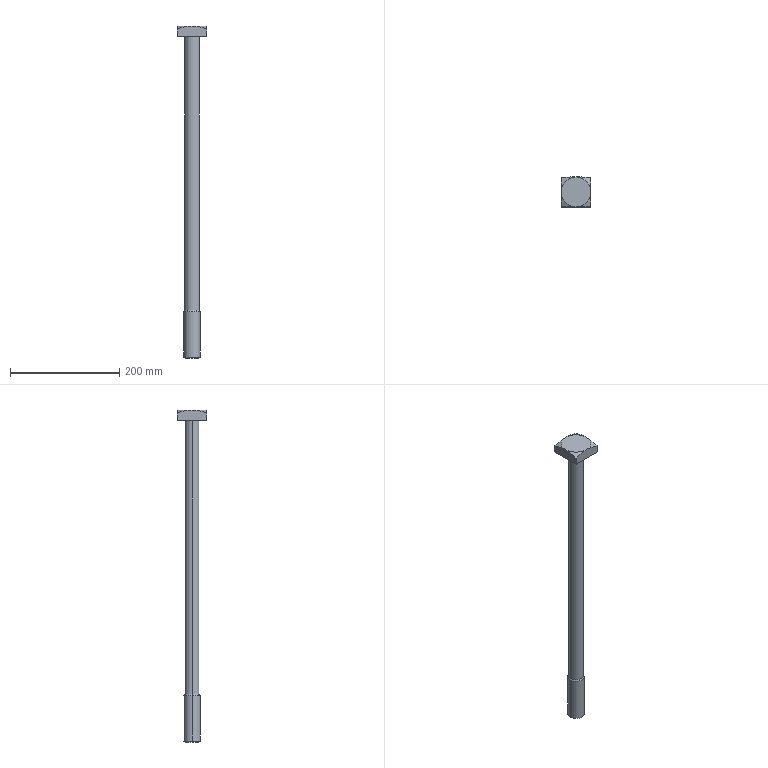Part | SolidWorks | features Cut 1, Extrusion 1, Fillet 1, LPattern 1, RevCut 1, Revolution 1 | 1 solid | 21 faces | box 55 x 55 x 609 mm | volume 405608 mm3 | cone 8 | plane 7 | cylinder 4 | torus 2 | commonest cylinder face diameters 27 x2 30 x2
STEP:
#1=CARTESIAN_POINT('',(11.969,0.,-590.));
#2=VERTEX_POINT('',#1);
#3=CARTESIAN_POINT('',(-11.969,0.,-590.));
#4=VERTEX_POINT('',#3);
#5=CARTESIAN_POINT('',(0.,0.,-590.));
#6=DIRECTION('',(0.,0.,1.));
#7=DIRECTION('',(1.,0.,0.));
#8=AXIS2_PLACEMENT_3D('',#5,#6,#7);
#9=CIRCLE('',#8,11.969);
#10=EDGE_CURVE('',#2,#4,#9,.T.);
#11=ORIENTED_EDGE('',*,*,#10,.T.);
#12=CARTESIAN_POINT('',(-15.,0.,-588.25));
#13=VERTEX_POINT('',#12);
#14=CARTESIAN_POINT('',(-11.969,0.,-590.));
#15=DIRECTION('',(-0.866,0.,0.5));
#16=VECTOR('',#15,1000.);
#17=LINE('',#14,#16);
#18=EDGE_CURVE('',#4,#13,#17,.T.);
#19=ORIENTED_EDGE('',*,*,#18,.T.);
#20=CARTESIAN_POINT('',(15.,0.,-588.25));
#21=VERTEX_POINT('',#20);
#22=CARTESIAN_POINT('',(0.,0.,-588.25));
#23=DIRECTION('',(0.,0.,1.));
#24=DIRECTION('',(1.,0.,0.));
#25=AXIS2_PLACEMENT_3D('',#22,#23,#24);
#26=CIRCLE('',#25,15.);
#27=EDGE_CURVE('',#21,#13,#26,.T.);
#28=ORIENTED_EDGE('',*,*,#27,.F.);
#29=CARTESIAN_POINT('',(11.969,0.,-590.));
#30=DIRECTION('',(0.866,0.,0.5));
#31=VECTOR('',#30,1000.);
#32=LINE('',#29,#31);
#33=EDGE_CURVE('',#2,#21,#32,.T.);
#34=ORIENTED_EDGE('',*,*,#33,.F.);
#35=EDGE_LOOP('',(#11,#19,#28,#34));
#36=FACE_OUTER_BOUND('',#35,.T.);
#37=CARTESIAN_POINT('',(0.,0.,-590.));
#38=DIRECTION('',(0.,0.,1.));
#39=DIRECTION('',(1.,0.,0.));
#40=AXIS2_PLACEMENT_3D('',#37,#38,#39);
#41=CONICAL_SURFACE('',#40,11.969,1.047);
#42=ADVANCED_FACE('',(#36),#41,.T.);
#43=CARTESIAN_POINT('',(-14.5,0.,0.));
#44=VERTEX_POINT('',#43);
#45=CARTESIAN_POINT('',(14.5,0.,0.));
#46=VERTEX_POINT('',#45);
#47=CARTESIAN_POINT('',(0.,0.,0.));
#48=DIRECTION('',(0.,0.,1.));
#49=DIRECTION('',(1.,0.,0.));
#50=AXIS2_PLACEMENT_3D('',#47,#48,#49);
#51=CIRCLE('',#50,14.5);
#52=EDGE_CURVE('',#44,#46,#51,.T.);
#53=ORIENTED_EDGE('',*,*,#52,.F.);
#54=CARTESIAN_POINT('',(-13.5,0.,-1.));
#55=VERTEX_POINT('',#54);
#56=CARTESIAN_POINT('',(-14.5,0.,-1.));
#57=DIRECTION('',(0.,1.,0.));
#58=DIRECTION('',(-1.,0.,0.));
#59=AXIS2_PLACEMENT_3D('',#56,#57,#58);
#60=CIRCLE('',#59,1.);
#61=EDGE_CURVE('',#44,#55,#60,.T.);
#62=ORIENTED_EDGE('',*,*,#61,.T.);
#63=CARTESIAN_POINT('',(13.5,0.,-1.));
#64=VERTEX_POINT('',#63);
#65=CARTESIAN_POINT('',(0.,0.,-1.));
#66=DIRECTION('',(0.,0.,-1.));
#67=DIRECTION('',(1.,0.,0.));
#68=AXIS2_PLACEMENT_3D('',#65,#66,#67);
#69=CIRCLE('',#68,13.5);
#70=EDGE_CURVE('',#64,#55,#69,.T.);
#71=ORIENTED_EDGE('',*,*,#70,.F.);
#72=CARTESIAN_POINT('',(14.5,0.,-1.));
#73=DIRECTION('',(0.,-1.,0.));
#74=DIRECTION('',(0.,0.,-1.));
#75=AXIS2_PLACEMENT_3D('',#72,#73,#74);
#76=CIRCLE('',#75,1.);
#77=EDGE_CURVE('',#46,#64,#76,.T.);
#78=ORIENTED_EDGE('',*,*,#77,.F.);
#79=EDGE_LOOP('',(#53,#62,#71,#78));
#80=FACE_OUTER_BOUND('',#79,.T.);
#81=CARTESIAN_POINT('',(0.,0.,-1.));
#82=DIRECTION('',(0.,0.,1.));
#83=DIRECTION('',(1.,0.,0.));
#84=AXIS2_PLACEMENT_3D('',#81,#82,#83);
#85=TOROIDAL_SURFACE('',#84,14.5,1.);
#86=ADVANCED_FACE('',(#80),#85,.F.);
#87=CARTESIAN_POINT('',(-15.,0.,-505.));
#88=VERTEX_POINT('',#87);
#89=CARTESIAN_POINT('',(15.,0.,-505.));
#90=VERTEX_POINT('',#89);
#91=CARTESIAN_POINT('',(0.,0.,-505.));
#92=DIRECTION('',(0.,0.,-1.));
#93=DIRECTION('',(-1.,0.,0.));
#94=AXIS2_PLACEMENT_3D('',#91,#92,#93);
#95=CIRCLE('',#94,15.);
#96=EDGE_CURVE('',#88,#90,#95,.T.);
#97=ORIENTED_EDGE('',*,*,#96,.T.);
#98=CARTESIAN_POINT('',(15.,0.,-590.));
#99=DIRECTION('',(0.,0.,-1.));
#100=VECTOR('',#99,1000.);
#101=LINE('',#98,#100);
#102=EDGE_CURVE('',#90,#21,#101,.T.);
#103=ORIENTED_EDGE('',*,*,#102,.T.);
#104=ORIENTED_EDGE('',*,*,#27,.T.);
#105=CARTESIAN_POINT('',(-15.,0.,-590.));
#106=DIRECTION('',(0.,0.,-1.));
#107=VECTOR('',#106,1000.);
#108=LINE('',#105,#107);
#109=EDGE_CURVE('',#88,#13,#108,.T.);
#110=ORIENTED_EDGE('',*,*,#109,.F.);
#111=EDGE_LOOP('',(#97,#103,#104,#110));
#112=FACE_OUTER_BOUND('',#111,.T.);
#113=CARTESIAN_POINT('',(0.,0.,-590.));
#114=DIRECTION('',(0.,0.,-1.));
#115=DIRECTION('',(-1.,0.,0.));
#116=AXIS2_PLACEMENT_3D('',#113,#114,#115);
#117=CYLINDRICAL_SURFACE('',#116,15.);
#118=ADVANCED_FACE('',(#112),#117,.T.);
#119=CARTESIAN_POINT('',(-13.5,0.,-502.402));
#120=VERTEX_POINT('',#119);
#121=CARTESIAN_POINT('',(13.5,0.,-502.402));
#122=VERTEX_POINT('',#121);
#123=CARTESIAN_POINT('',(0.,0.,-502.402));
#124=DIRECTION('',(0.,0.,-1.));
#125=DIRECTION('',(-1.,0.,0.));
#126=AXIS2_PLACEMENT_3D('',#123,#124,#125);
#127=CIRCLE('',#126,13.5);
#128=EDGE_CURVE('',#120,#122,#127,.T.);
#129=ORIENTED_EDGE('',*,*,#128,.T.);
#130=CARTESIAN_POINT('',(13.5,0.,-502.402));
#131=DIRECTION('',(0.5,0.,-0.866));
#132=VECTOR('',#131,1000.);
#133=LINE('',#130,#132);
#134=EDGE_CURVE('',#122,#90,#133,.T.);
#135=ORIENTED_EDGE('',*,*,#134,.T.);
#136=ORIENTED_EDGE('',*,*,#96,.F.);
#137=CARTESIAN_POINT('',(-13.5,0.,-502.402));
#138=DIRECTION('',(-0.5,0.,-0.866));
#139=VECTOR('',#138,1000.);
#140=LINE('',#137,#139);
#141=EDGE_CURVE('',#120,#88,#140,.T.);
#142=ORIENTED_EDGE('',*,*,#141,.F.);
#143=EDGE_LOOP('',(#129,#135,#136,#142));
#144=FACE_OUTER_BOUND('',#143,.T.);
#145=CARTESIAN_POINT('',(0.,0.,-502.402));
#146=DIRECTION('',(0.,0.,-1.));
#147=DIRECTION('',(-1.,0.,0.));
#148=AXIS2_PLACEMENT_3D('',#145,#146,#147);
#149=CONICAL_SURFACE('',#148,13.5,0.5236);
#150=ADVANCED_FACE('',(#144),#149,.T.);
#151=CARTESIAN_POINT('',(0.,0.,-1.));
#152=DIRECTION('',(0.,0.,-1.));
#153=DIRECTION('',(1.,0.,0.));
#154=AXIS2_PLACEMENT_3D('',#151,#152,#153);
#155=CIRCLE('',#154,13.5);
#156=EDGE_CURVE('',#55,#64,#155,.T.);
#157=ORIENTED_EDGE('',*,*,#156,.T.);
#158=CARTESIAN_POINT('',(13.5,0.,-590.));
#159=DIRECTION('',(0.,0.,-1.));
#160=VECTOR('',#159,1000.);
#161=LINE('',#158,#160);
#162=EDGE_CURVE('',#64,#122,#161,.T.);
#163=ORIENTED_EDGE('',*,*,#162,.T.);
#164=ORIENTED_EDGE('',*,*,#128,.F.);
#165=CARTESIAN_POINT('',(-13.5,0.,-590.));
#166=DIRECTION('',(0.,0.,-1.));
#167=VECTOR('',#166,1000.);
#168=LINE('',#165,#167);
#169=EDGE_CURVE('',#55,#120,#168,.T.);
#170=ORIENTED_EDGE('',*,*,#169,.F.);
#171=EDGE_LOOP('',(#157,#163,#164,#170));
#172=FACE_OUTER_BOUND('',#171,.T.);
#173=CARTESIAN_POINT('',(0.,0.,-590.));
#174=DIRECTION('',(0.,0.,-1.));
#175=DIRECTION('',(-1.,0.,0.));
#176=AXIS2_PLACEMENT_3D('',#173,#174,#175);
#177=CYLINDRICAL_SURFACE('',#176,13.5);
#178=ADVANCED_FACE('',(#172),#177,.T.);
#179=CARTESIAN_POINT('',(0.,0.,0.));
#180=DIRECTION('',(0.,0.,1.));
#181=DIRECTION('',(1.,0.,0.));
#182=AXIS2_PLACEMENT_3D('',#179,#180,#181);
#183=CIRCLE('',#182,14.5);
#184=EDGE_CURVE('',#46,#44,#183,.T.);
#185=ORIENTED_EDGE('',*,*,#184,.T.);
#186=ORIENTED_EDGE('',*,*,#52,.T.);
#187=EDGE_LOOP('',(#185,#186));
#188=FACE_BOUND('',#187,.T.);
#189=CARTESIAN_POINT('',(-27.5,27.5,0.));
#190=VERTEX_POINT('',#189);
#191=CARTESIAN_POINT('',(-27.5,-27.5,0.));
#192=VERTEX_POINT('',#191);
#193=CARTESIAN_POINT('',(-27.5,27.5,0.));
#194=DIRECTION('',(0.,-1.,0.));
#195=VECTOR('',#194,1000.);
#196=LINE('',#193,#195);
#197=EDGE_CURVE('',#190,#192,#196,.T.);
#198=ORIENTED_EDGE('',*,*,#197,.F.);
#199=CARTESIAN_POINT('',(27.5,27.5,0.));
#200=VERTEX_POINT('',#199);
#201=CARTESIAN_POINT('',(-27.5,27.5,0.));
#202=DIRECTION('',(-1.,0.,0.));
#203=VECTOR('',#202,1000.);
#204=LINE('',#201,#203);
#205=EDGE_CURVE('',#200,#190,#204,.T.);
#206=ORIENTED_EDGE('',*,*,#205,.F.);
#207=CARTESIAN_POINT('',(27.5,-27.5,0.));
#208=VERTEX_POINT('',#207);
#209=CARTESIAN_POINT('',(27.5,27.5,0.));
#210=DIRECTION('',(0.,1.,0.));
#211=VECTOR('',#210,1000.);
#212=LINE('',#209,#211);
#213=EDGE_CURVE('',#208,#200,#212,.T.);
#214=ORIENTED_EDGE('',*,*,#213,.F.);
#215=CARTESIAN_POINT('',(-27.5,-27.5,0.));
#216=DIRECTION('',(1.,0.,0.));
#217=VECTOR('',#216,1000.);
#218=LINE('',#215,#217);
#219=EDGE_CURVE('',#192,#208,#218,.T.);
#220=ORIENTED_EDGE('',*,*,#219,.F.);
#221=EDGE_LOOP('',(#198,#206,#214,#220));
#222=FACE_OUTER_BOUND('',#221,.T.);
#223=CARTESIAN_POINT('',(-27.5,-27.5,0.));
#224=DIRECTION('',(0.,0.,1.));
#225=DIRECTION('',(1.,0.,0.));
#226=AXIS2_PLACEMENT_3D('',#223,#224,#225);
#227=PLANE('',#226);
#228=ADVANCED_FACE('',(#188,#222),#227,.F.);
#229=CARTESIAN_POINT('',(-27.5,27.5,13.688));
#230=VERTEX_POINT('',#229);
#231=CARTESIAN_POINT('',(-27.5,0.,19.));
#232=VERTEX_POINT('',#231);
#233=CARTESIAN_POINT('',(-27.5,27.5,13.688));
#234=CARTESIAN_POINT('',(-27.5,25.285,14.419));
#235=CARTESIAN_POINT('',(-27.5,23.059,15.109));
#236=CARTESIAN_POINT('',(-27.5,18.569,16.373));
#237=CARTESIAN_POINT('',(-27.5,16.306,16.946));
#238=CARTESIAN_POINT('',(-27.5,11.727,17.915));
#239=CARTESIAN_POINT('',(-27.5,9.41,18.312));
#240=CARTESIAN_POINT('',(-27.5,6.466,18.653));
#241=CARTESIAN_POINT('',(-27.5,5.875,18.713));
#242=CARTESIAN_POINT('',(-27.5,4.695,18.817));
#243=CARTESIAN_POINT('',(-27.5,4.105,18.861));
#244=CARTESIAN_POINT('',(-27.5,2.341,18.965));
#245=CARTESIAN_POINT('',(-27.5,1.169,19.));
#246=CARTESIAN_POINT('',(-27.5,0.,19.));
#247=B_SPLINE_CURVE_WITH_KNOTS('',3,(#233,#234,#235,#236,#237,#238,#239,#240,#241,#242,#243,#244,#245,#246),.UNSPECIFIED.,.F.,.F.,(4,2,2,2,2,2,4),(0.02351,0.0305,0.03749,0.04449,0.04624,0.04799,0.05148),.UNSPECIFIED.);
#248=EDGE_CURVE('',#230,#232,#247,.T.);
#249=ORIENTED_EDGE('',*,*,#248,.F.);
#250=CARTESIAN_POINT('',(-27.5,27.5,19.));
#251=DIRECTION('',(0.,0.,-1.));
#252=VECTOR('',#251,1000.);
#253=LINE('',#250,#252);
#254=EDGE_CURVE('',#230,#190,#253,.T.);
#255=ORIENTED_EDGE('',*,*,#254,.T.);
#256=ORIENTED_EDGE('',*,*,#197,.T.);
#257=CARTESIAN_POINT('',(-27.5,-27.5,13.688));
#258=VERTEX_POINT('',#257);
#259=CARTESIAN_POINT('',(-27.5,-27.5,19.));
#260=DIRECTION('',(0.,0.,-1.));
#261=VECTOR('',#260,1000.);
#262=LINE('',#259,#261);
#263=EDGE_CURVE('',#258,#192,#262,.T.);
#264=ORIENTED_EDGE('',*,*,#263,.F.);
#265=CARTESIAN_POINT('',(-27.5,0.,19.));
#266=CARTESIAN_POINT('',(-27.5,-2.343,19.));
#267=CARTESIAN_POINT('',(-27.5,-4.671,18.858));
#268=CARTESIAN_POINT('',(-27.5,-9.3,18.327));
#269=CARTESIAN_POINT('',(-27.5,-11.601,17.938));
#270=CARTESIAN_POINT('',(-27.5,-16.182,16.975));
#271=CARTESIAN_POINT('',(-27.5,-18.462,16.401));
#272=CARTESIAN_POINT('',(-27.5,-23.009,15.125));
#273=CARTESIAN_POINT('',(-27.5,-25.262,14.426));
#274=CARTESIAN_POINT('',(-27.5,-27.5,13.688));
#275=B_SPLINE_CURVE_WITH_KNOTS('',3,(#265,#266,#267,#268,#269,#270,#271,#272,#273,#274),.UNSPECIFIED.,.F.,.F.,(4,2,2,2,4),(0.05148,0.0585,0.06551,0.07252,0.07953),.UNSPECIFIED.);
#276=EDGE_CURVE('',#232,#258,#275,.T.);
#277=ORIENTED_EDGE('',*,*,#276,.F.);
#278=EDGE_LOOP('',(#249,#255,#256,#264,#277));
#279=FACE_OUTER_BOUND('',#278,.T.);
#280=CARTESIAN_POINT('',(-27.5,27.5,19.));
#281=DIRECTION('',(1.,0.,0.));
#282=DIRECTION('',(0.,1.,0.));
#283=AXIS2_PLACEMENT_3D('',#280,#281,#282);
#284=PLANE('',#283);
#285=ADVANCED_FACE('',(#279),#284,.F.);
#286=CARTESIAN_POINT('',(0.,-27.5,19.));
#287=VERTEX_POINT('',#286);
#288=CARTESIAN_POINT('',(-27.5,-27.5,13.688));
#289=CARTESIAN_POINT('',(-25.262,-27.5,14.426));
#290=CARTESIAN_POINT('',(-23.009,-27.5,15.125));
#291=CARTESIAN_POINT('',(-18.462,-27.5,16.401));
#292=CARTESIAN_POINT('',(-16.182,-27.5,16.975));
#293=CARTESIAN_POINT('',(-11.601,-27.5,17.938));
#294=CARTESIAN_POINT('',(-9.3,-27.5,18.327));
#295=CARTESIAN_POINT('',(-4.671,-27.5,18.858));
#296=CARTESIAN_POINT('',(-2.343,-27.5,19.));
#297=CARTESIAN_POINT('',(0.,-27.5,19.));
#298=B_SPLINE_CURVE_WITH_KNOTS('',3,(#288,#289,#290,#291,#292,#293,#294,#295,#296,#297),.UNSPECIFIED.,.F.,.F.,(4,2,2,2,4),(0.02964,0.0367,0.04377,0.05083,0.0579),.UNSPECIFIED.);
#299=EDGE_CURVE('',#258,#287,#298,.T.);
#300=ORIENTED_EDGE('',*,*,#299,.F.);
#301=ORIENTED_EDGE('',*,*,#263,.T.);
#302=ORIENTED_EDGE('',*,*,#219,.T.);
#303=CARTESIAN_POINT('',(27.5,-27.5,13.688));
#304=VERTEX_POINT('',#303);
#305=CARTESIAN_POINT('',(27.5,-27.5,19.));
#306=DIRECTION('',(0.,0.,-1.));
#307=VECTOR('',#306,1000.);
#308=LINE('',#305,#307);
#309=EDGE_CURVE('',#304,#208,#308,.T.);
#310=ORIENTED_EDGE('',*,*,#309,.F.);
#311=CARTESIAN_POINT('',(0.,-27.5,19.));
#312=CARTESIAN_POINT('',(1.169,-27.5,19.));
#313=CARTESIAN_POINT('',(2.341,-27.5,18.965));
#314=CARTESIAN_POINT('',(4.105,-27.5,18.861));
#315=CARTESIAN_POINT('',(4.695,-27.5,18.817));
#316=CARTESIAN_POINT('',(5.875,-27.5,18.713));
#317=CARTESIAN_POINT('',(6.466,-27.5,18.653));
#318=CARTESIAN_POINT('',(9.41,-27.5,18.312));
#319=CARTESIAN_POINT('',(11.727,-27.5,17.915));
#320=CARTESIAN_POINT('',(16.306,-27.5,16.946));
#321=CARTESIAN_POINT('',(18.569,-27.5,16.373));
#322=CARTESIAN_POINT('',(23.059,-27.5,15.109));
#323=CARTESIAN_POINT('',(25.285,-27.5,14.419));
#324=CARTESIAN_POINT('',(27.5,-27.5,13.688));
#325=B_SPLINE_CURVE_WITH_KNOTS('',3,(#311,#312,#313,#314,#315,#316,#317,#318,#319,#320,#321,#322,#323,#324),.UNSPECIFIED.,.F.,.F.,(4,2,2,2,2,2,4),(0.0579,0.06142,0.06318,0.06494,0.07199,0.07903,0.08608),.UNSPECIFIED.);
#326=EDGE_CURVE('',#287,#304,#325,.T.);
#327=ORIENTED_EDGE('',*,*,#326,.F.);
#328=EDGE_LOOP('',(#300,#301,#302,#310,#327));
#329=FACE_OUTER_BOUND('',#328,.T.);
#330=CARTESIAN_POINT('',(-27.5,-27.5,19.));
#331=DIRECTION('',(0.,1.,0.));
#332=DIRECTION('',(0.,0.,1.));
#333=AXIS2_PLACEMENT_3D('',#330,#331,#332);
#334=PLANE('',#333);
#335=ADVANCED_FACE('',(#329),#334,.F.);
#336=CARTESIAN_POINT('',(27.5,0.,19.));
#337=VERTEX_POINT('',#336);
#338=CARTESIAN_POINT('',(27.5,-27.5,13.688));
#339=CARTESIAN_POINT('',(27.5,-25.262,14.426));
#340=CARTESIAN_POINT('',(27.5,-23.009,15.125));
#341=CARTESIAN_POINT('',(27.5,-18.462,16.401));
#342=CARTESIAN_POINT('',(27.5,-16.182,16.975));
#343=CARTESIAN_POINT('',(27.5,-11.601,17.938));
#344=CARTESIAN_POINT('',(27.5,-9.3,18.327));
#345=CARTESIAN_POINT('',(27.5,-4.671,18.858));
#346=CARTESIAN_POINT('',(27.5,-2.343,19.));
#347=CARTESIAN_POINT('',(27.5,0.,19.));
#348=B_SPLINE_CURVE_WITH_KNOTS('',3,(#338,#339,#340,#341,#342,#343,#344,#345,#346,#347),.UNSPECIFIED.,.F.,.F.,(4,2,2,2,4),(0.02964,0.0367,0.04377,0.05083,0.0579),.UNSPECIFIED.);
#349=EDGE_CURVE('',#304,#337,#348,.T.);
#350=ORIENTED_EDGE('',*,*,#349,.F.);
#351=ORIENTED_EDGE('',*,*,#309,.T.);
#352=ORIENTED_EDGE('',*,*,#213,.T.);
#353=CARTESIAN_POINT('',(27.5,27.5,13.688));
#354=VERTEX_POINT('',#353);
#355=CARTESIAN_POINT('',(27.5,27.5,19.));
#356=DIRECTION('',(0.,0.,-1.));
#357=VECTOR('',#356,1000.);
#358=LINE('',#355,#357);
#359=EDGE_CURVE('',#354,#200,#358,.T.);
#360=ORIENTED_EDGE('',*,*,#359,.F.);
#361=CARTESIAN_POINT('',(27.5,0.,19.));
#362=CARTESIAN_POINT('',(27.5,1.169,19.));
#363=CARTESIAN_POINT('',(27.5,2.341,18.965));
#364=CARTESIAN_POINT('',(27.5,4.105,18.861));
#365=CARTESIAN_POINT('',(27.5,4.695,18.817));
#366=CARTESIAN_POINT('',(27.5,5.875,18.713));
#367=CARTESIAN_POINT('',(27.5,6.466,18.653));
#368=CARTESIAN_POINT('',(27.5,9.41,18.312));
#369=CARTESIAN_POINT('',(27.5,11.727,17.915));
#370=CARTESIAN_POINT('',(27.5,16.306,16.946));
#371=CARTESIAN_POINT('',(27.5,18.569,16.373));
#372=CARTESIAN_POINT('',(27.5,23.059,15.109));
#373=CARTESIAN_POINT('',(27.5,25.285,14.419));
#374=CARTESIAN_POINT('',(27.5,27.5,13.688));
#375=B_SPLINE_CURVE_WITH_KNOTS('',3,(#361,#362,#363,#364,#365,#366,#367,#368,#369,#370,#371,#372,#373,#374),.UNSPECIFIED.,.F.,.F.,(4,2,2,2,2,2,4),(0.0579,0.06142,0.06318,0.06494,0.07199,0.07903,0.08608),.UNSPECIFIED.);
#376=EDGE_CURVE('',#337,#354,#375,.T.);
#377=ORIENTED_EDGE('',*,*,#376,.F.);
#378=EDGE_LOOP('',(#350,#351,#352,#360,#377));
#379=FACE_OUTER_BOUND('',#378,.T.);
#380=CARTESIAN_POINT('',(27.5,27.5,19.));
#381=DIRECTION('',(-1.,0.,0.));
#382=DIRECTION('',(0.,0.,1.));
#383=AXIS2_PLACEMENT_3D('',#380,#381,#382);
#384=PLANE('',#383);
#385=ADVANCED_FACE('',(#379),#384,.F.);
#386=CARTESIAN_POINT('',(0.,27.5,19.));
#387=VERTEX_POINT('',#386);
#388=CARTESIAN_POINT('',(27.5,27.5,13.688));
#389=CARTESIAN_POINT('',(25.285,27.5,14.419));
#390=CARTESIAN_POINT('',(23.059,27.5,15.109));
#391=CARTESIAN_POINT('',(18.569,27.5,16.373));
#392=CARTESIAN_POINT('',(16.306,27.5,16.946));
#393=CARTESIAN_POINT('',(11.727,27.5,17.915));
#394=CARTESIAN_POINT('',(9.41,27.5,18.312));
#395=CARTESIAN_POINT('',(6.466,27.5,18.653));
#396=CARTESIAN_POINT('',(5.875,27.5,18.713));
#397=CARTESIAN_POINT('',(4.695,27.5,18.817));
#398=CARTESIAN_POINT('',(4.105,27.5,18.861));
#399=CARTESIAN_POINT('',(2.341,27.5,18.965));
#400=CARTESIAN_POINT('',(1.169,27.5,19.));
#401=CARTESIAN_POINT('',(0.,27.5,19.));
#402=B_SPLINE_CURVE_WITH_KNOTS('',3,(#388,#389,#390,#391,#392,#393,#394,#395,#396,#397,#398,#399,#400,#401),.UNSPECIFIED.,.F.,.F.,(4,2,2,2,2,2,4),(0.02351,0.0305,0.03749,0.04449,0.04624,0.04799,0.05148),.UNSPECIFIED.);
#403=EDGE_CURVE('',#354,#387,#402,.T.);
#404=ORIENTED_EDGE('',*,*,#403,.F.);
#405=ORIENTED_EDGE('',*,*,#359,.T.);
#406=ORIENTED_EDGE('',*,*,#205,.T.);
#407=ORIENTED_EDGE('',*,*,#254,.F.);
#408=CARTESIAN_POINT('',(0.,27.5,19.));
#409=CARTESIAN_POINT('',(-2.343,27.5,19.));
#410=CARTESIAN_POINT('',(-4.671,27.5,18.858));
#411=CARTESIAN_POINT('',(-9.3,27.5,18.327));
#412=CARTESIAN_POINT('',(-11.601,27.5,17.938));
#413=CARTESIAN_POINT('',(-16.182,27.5,16.975));
#414=CARTESIAN_POINT('',(-18.462,27.5,16.401));
#415=CARTESIAN_POINT('',(-23.009,27.5,15.125));
#416=CARTESIAN_POINT('',(-25.262,27.5,14.426));
#417=CARTESIAN_POINT('',(-27.5,27.5,13.688));
#418=B_SPLINE_CURVE_WITH_KNOTS('',3,(#408,#409,#410,#411,#412,#413,#414,#415,#416,#417),.UNSPECIFIED.,.F.,.F.,(4,2,2,2,4),(0.05148,0.0585,0.06551,0.07252,0.07953),.UNSPECIFIED.);
#419=EDGE_CURVE('',#387,#230,#418,.T.);
#420=ORIENTED_EDGE('',*,*,#419,.F.);
#421=EDGE_LOOP('',(#404,#405,#406,#407,#420));
#422=FACE_OUTER_BOUND('',#421,.T.);
#423=CARTESIAN_POINT('',(-27.5,27.5,19.));
#424=DIRECTION('',(0.,-1.,0.));
#425=DIRECTION('',(0.,0.,-1.));
#426=AXIS2_PLACEMENT_3D('',#423,#424,#425);
#427=PLANE('',#426);
#428=ADVANCED_FACE('',(#422),#427,.F.);
#429=ORIENTED_EDGE('',*,*,#326,.T.);
#430=ORIENTED_EDGE('',*,*,#349,.T.);
#431=CARTESIAN_POINT('',(0.,0.,19.));
#432=DIRECTION('',(0.,0.,1.));
#433=DIRECTION('',(1.,0.,0.));
#434=AXIS2_PLACEMENT_3D('',#431,#432,#433);
#435=CIRCLE('',#434,27.5);
#436=EDGE_CURVE('',#287,#337,#435,.T.);
#437=ORIENTED_EDGE('',*,*,#436,.F.);
#438=EDGE_LOOP('',(#429,#430,#437));
#439=FACE_OUTER_BOUND('',#438,.T.);
#440=CARTESIAN_POINT('',(0.,0.,19.));
#441=DIRECTION('',(0.,0.,-1.));
#442=DIRECTION('',(1.,0.,0.));
#443=AXIS2_PLACEMENT_3D('',#440,#441,#442);
#444=CONICAL_SURFACE('',#443,27.5,1.134);
#445=ADVANCED_FACE('',(#439),#444,.T.);
#446=ORIENTED_EDGE('',*,*,#276,.T.);
#447=ORIENTED_EDGE('',*,*,#299,.T.);
#448=CARTESIAN_POINT('',(0.,0.,19.));
#449=DIRECTION('',(0.,0.,1.));
#450=DIRECTION('',(1.,0.,0.));
#451=AXIS2_PLACEMENT_3D('',#448,#449,#450);
#452=CIRCLE('',#451,27.5);
#453=EDGE_CURVE('',#232,#287,#452,.T.);
#454=ORIENTED_EDGE('',*,*,#453,.F.);
#455=EDGE_LOOP('',(#446,#447,#454));
#456=FACE_OUTER_BOUND('',#455,.T.);
#457=CARTESIAN_POINT('',(0.,0.,19.));
#458=DIRECTION('',(0.,0.,-1.));
#459=DIRECTION('',(1.,0.,0.));
#460=AXIS2_PLACEMENT_3D('',#457,#458,#459);
#461=CONICAL_SURFACE('',#460,27.5,1.134);
#462=ADVANCED_FACE('',(#456),#461,.T.);
#463=ORIENTED_EDGE('',*,*,#248,.T.);
#464=CARTESIAN_POINT('',(0.,0.,19.));
#465=DIRECTION('',(0.,0.,1.));
#466=DIRECTION('',(1.,0.,0.));
#467=AXIS2_PLACEMENT_3D('',#464,#465,#466);
#468=CIRCLE('',#467,27.5);
#469=EDGE_CURVE('',#387,#232,#468,.T.);
#470=ORIENTED_EDGE('',*,*,#469,.F.);
#471=ORIENTED_EDGE('',*,*,#419,.T.);
#472=EDGE_LOOP('',(#463,#470,#471));
#473=FACE_OUTER_BOUND('',#472,.T.);
#474=CARTESIAN_POINT('',(0.,0.,19.));
#475=DIRECTION('',(0.,0.,-1.));
#476=DIRECTION('',(1.,0.,0.));
#477=AXIS2_PLACEMENT_3D('',#474,#475,#476);
#478=CONICAL_SURFACE('',#477,27.5,1.134);
#479=ADVANCED_FACE('',(#473),#478,.T.);
#480=ORIENTED_EDGE('',*,*,#376,.T.);
#481=ORIENTED_EDGE('',*,*,#403,.T.);
#482=CARTESIAN_POINT('',(0.,0.,19.));
#483=DIRECTION('',(0.,0.,1.));
#484=DIRECTION('',(1.,0.,0.));
#485=AXIS2_PLACEMENT_3D('',#482,#483,#484);
#486=CIRCLE('',#485,27.5);
#487=EDGE_CURVE('',#337,#387,#486,.T.);
#488=ORIENTED_EDGE('',*,*,#487,.F.);
#489=EDGE_LOOP('',(#480,#481,#488));
#490=FACE_OUTER_BOUND('',#489,.T.);
#491=CARTESIAN_POINT('',(0.,0.,19.));
#492=DIRECTION('',(0.,0.,-1.));
#493=DIRECTION('',(1.,0.,0.));
#494=AXIS2_PLACEMENT_3D('',#491,#492,#493);
#495=CONICAL_SURFACE('',#494,27.5,1.134);
#496=ADVANCED_FACE('',(#490),#495,.T.);
#497=ORIENTED_EDGE('',*,*,#436,.T.);
#498=ORIENTED_EDGE('',*,*,#487,.T.);
#499=ORIENTED_EDGE('',*,*,#469,.T.);
#500=ORIENTED_EDGE('',*,*,#453,.T.);
#501=EDGE_LOOP('',(#497,#498,#499,#500));
#502=FACE_OUTER_BOUND('',#501,.T.);
#503=CARTESIAN_POINT('',(-27.5,-27.5,19.));
#504=DIRECTION('',(0.,0.,1.));
#505=DIRECTION('',(1.,0.,0.));
#506=AXIS2_PLACEMENT_3D('',#503,#504,#505);
#507=PLANE('',#506);
#508=ADVANCED_FACE('',(#502),#507,.T.);
#509=ORIENTED_EDGE('',*,*,#162,.F.);
#510=ORIENTED_EDGE('',*,*,#70,.T.);
#511=ORIENTED_EDGE('',*,*,#169,.T.);
#512=CARTESIAN_POINT('',(0.,0.,-502.402));
#513=DIRECTION('',(0.,0.,-1.));
#514=DIRECTION('',(-1.,0.,0.));
#515=AXIS2_PLACEMENT_3D('',#512,#513,#514);
#516=CIRCLE('',#515,13.5);
#517=EDGE_CURVE('',#122,#120,#516,.T.);
#518=ORIENTED_EDGE('',*,*,#517,.F.);
#519=EDGE_LOOP('',(#509,#510,#511,#518));
#520=FACE_OUTER_BOUND('',#519,.T.);
#521=CARTESIAN_POINT('',(0.,0.,-590.));
#522=DIRECTION('',(0.,0.,-1.));
#523=DIRECTION('',(-1.,0.,0.));
#524=AXIS2_PLACEMENT_3D('',#521,#522,#523);
#525=CYLINDRICAL_SURFACE('',#524,13.5);
#526=ADVANCED_FACE('',(#520),#525,.T.);
#527=ORIENTED_EDGE('',*,*,#134,.F.);
#528=ORIENTED_EDGE('',*,*,#517,.T.);
#529=ORIENTED_EDGE('',*,*,#141,.T.);
#530=CARTESIAN_POINT('',(0.,0.,-505.));
#531=DIRECTION('',(0.,0.,-1.));
#532=DIRECTION('',(-1.,0.,0.));
#533=AXIS2_PLACEMENT_3D('',#530,#531,#532);
#534=CIRCLE('',#533,15.);
#535=EDGE_CURVE('',#90,#88,#534,.T.);
#536=ORIENTED_EDGE('',*,*,#535,.F.);
#537=EDGE_LOOP('',(#527,#528,#529,#536));
#538=FACE_OUTER_BOUND('',#537,.T.);
#539=CARTESIAN_POINT('',(0.,0.,-502.402));
#540=DIRECTION('',(0.,0.,-1.));
#541=DIRECTION('',(-1.,0.,0.));
#542=AXIS2_PLACEMENT_3D('',#539,#540,#541);
#543=CONICAL_SURFACE('',#542,13.5,0.5236);
#544=ADVANCED_FACE('',(#538),#543,.T.);
#545=ORIENTED_EDGE('',*,*,#102,.F.);
#546=ORIENTED_EDGE('',*,*,#535,.T.);
#547=ORIENTED_EDGE('',*,*,#109,.T.);
#548=CARTESIAN_POINT('',(0.,0.,-588.25));
#549=DIRECTION('',(0.,0.,1.));
#550=DIRECTION('',(1.,0.,0.));
#551=AXIS2_PLACEMENT_3D('',#548,#549,#550);
#552=CIRCLE('',#551,15.);
#553=EDGE_CURVE('',#13,#21,#552,.T.);
#554=ORIENTED_EDGE('',*,*,#553,.T.);
#555=EDGE_LOOP('',(#545,#546,#547,#554));
#556=FACE_OUTER_BOUND('',#555,.T.);
#557=CARTESIAN_POINT('',(0.,0.,-590.));
#558=DIRECTION('',(0.,0.,-1.));
#559=DIRECTION('',(-1.,0.,0.));
#560=AXIS2_PLACEMENT_3D('',#557,#558,#559);
#561=CYLINDRICAL_SURFACE('',#560,15.);
#562=ADVANCED_FACE('',(#556),#561,.T.);
#563=ORIENTED_EDGE('',*,*,#61,.F.);
#564=ORIENTED_EDGE('',*,*,#184,.F.);
#565=ORIENTED_EDGE('',*,*,#77,.T.);
#566=ORIENTED_EDGE('',*,*,#156,.F.);
#567=EDGE_LOOP('',(#563,#564,#565,#566));
#568=FACE_OUTER_BOUND('',#567,.T.);
#569=CARTESIAN_POINT('',(0.,0.,-1.));
#570=DIRECTION('',(0.,0.,1.));
#571=DIRECTION('',(1.,0.,0.));
#572=AXIS2_PLACEMENT_3D('',#569,#570,#571);
#573=TOROIDAL_SURFACE('',#572,14.5,1.);
#574=ADVANCED_FACE('',(#568),#573,.F.);
#575=ORIENTED_EDGE('',*,*,#18,.F.);
#576=CARTESIAN_POINT('',(0.,0.,-590.));
#577=DIRECTION('',(0.,0.,1.));
#578=DIRECTION('',(1.,0.,0.));
#579=AXIS2_PLACEMENT_3D('',#576,#577,#578);
#580=CIRCLE('',#579,11.969);
#581=EDGE_CURVE('',#4,#2,#580,.T.);
#582=ORIENTED_EDGE('',*,*,#581,.T.);
#583=ORIENTED_EDGE('',*,*,#33,.T.);
#584=ORIENTED_EDGE('',*,*,#553,.F.);
#585=EDGE_LOOP('',(#575,#582,#583,#584));
#586=FACE_OUTER_BOUND('',#585,.T.);
#587=CARTESIAN_POINT('',(0.,0.,-590.));
#588=DIRECTION('',(0.,0.,1.));
#589=DIRECTION('',(1.,0.,0.));
#590=AXIS2_PLACEMENT_3D('',#587,#588,#589);
#591=CONICAL_SURFACE('',#590,11.969,1.047);
#592=ADVANCED_FACE('',(#586),#591,.T.);
#593=ORIENTED_EDGE('',*,*,#10,.F.);
#594=ORIENTED_EDGE('',*,*,#581,.F.);
#595=EDGE_LOOP('',(#593,#594));
#596=FACE_OUTER_BOUND('',#595,.T.);
#597=CARTESIAN_POINT('',(15.,0.,-590.));
#598=DIRECTION('',(0.,0.,1.));
#599=DIRECTION('',(1.,0.,0.));
#600=AXIS2_PLACEMENT_3D('',#597,#598,#599);
#601=PLANE('',#600);
#602=ADVANCED_FACE('',(#596),#601,.F.);
#603=CLOSED_SHELL('',(#42,#86,#118,#150,#178,#228,#285,#335,#385,#428,#445,#462,#479,#496,#508,#526,#544,#562,#574,#592,#602));
#604=MANIFOLD_SOLID_BREP('',#603);
#605=CARTESIAN_POINT('',(0.,0.,0.));
#606=DIRECTION('',(0.,0.,1.));
#607=DIRECTION('',(1.,0.,0.));
#608=AXIS2_PLACEMENT_3D('',#605,#606,#607);
#609=(LENGTH_UNIT()NAMED_UNIT(*)SI_UNIT(.MILLI.,.METRE.));
#610=UNCERTAINTY_MEASURE_WITH_UNIT(LENGTH_MEASURE(0.00001),#609,'','');
#611=(NAMED_UNIT(*)PLANE_ANGLE_UNIT()SI_UNIT($,.RADIAN.));
#612=(NAMED_UNIT(*)SI_UNIT($,.STERADIAN.)SOLID_ANGLE_UNIT());
#613=(GEOMETRIC_REPRESENTATION_CONTEXT(3)GLOBAL_UNCERTAINTY_ASSIGNED_CONTEXT((#610))GLOBAL_UNIT_ASSIGNED_CONTEXT((#609,#611,#612))REPRESENTATION_CONTEXT('',''));
#614=ADVANCED_BREP_SHAPE_REPRESENTATION('',(#604,#608),#613);